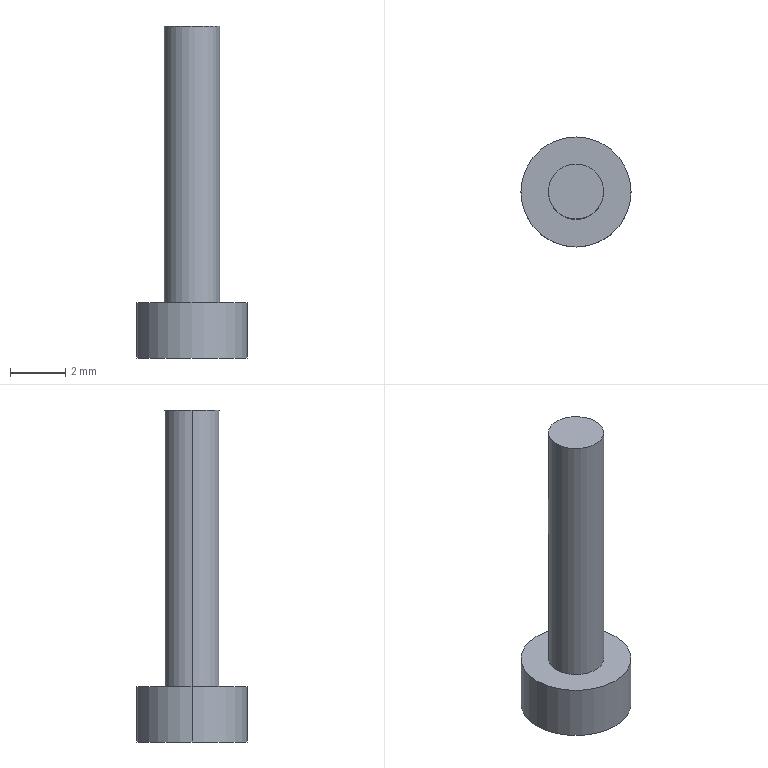Part | SolidWorks | features BaseBody 1 | 1 solid | 14 faces | box 3.98 x 3.98 x 12 mm | volume 54.19 mm3 | plane 10 | cylinder 4 | commonest cylinder face diameters 2 x2 3.98 x2
STEP:
#1=CARTESIAN_POINT('',(-1.,0.,12.));
#2=VERTEX_POINT('',#1);
#3=CARTESIAN_POINT('',(1.,0.,12.));
#4=VERTEX_POINT('',#3);
#5=CARTESIAN_POINT('',(0.,0.,12.));
#6=DIRECTION('',(0.,0.,-1.));
#7=DIRECTION('',(-1.,0.,0.));
#8=AXIS2_PLACEMENT_3D('',#5,#6,#7);
#9=CIRCLE('',#8,1.);
#10=EDGE_CURVE('',#2,#4,#9,.T.);
#11=ORIENTED_EDGE('',*,*,#10,.T.);
#12=CARTESIAN_POINT('',(1.,0.,2.));
#13=VERTEX_POINT('',#12);
#14=CARTESIAN_POINT('',(1.,0.,12.));
#15=DIRECTION('',(0.,0.,-1.));
#16=VECTOR('',#15,1000.);
#17=LINE('',#14,#16);
#18=EDGE_CURVE('',#4,#13,#17,.T.);
#19=ORIENTED_EDGE('',*,*,#18,.T.);
#20=CARTESIAN_POINT('',(-1.,0.,2.));
#21=VERTEX_POINT('',#20);
#22=CARTESIAN_POINT('',(0.,0.,2.));
#23=DIRECTION('',(0.,0.,1.));
#24=DIRECTION('',(-1.,0.,0.));
#25=AXIS2_PLACEMENT_3D('',#22,#23,#24);
#26=CIRCLE('',#25,1.);
#27=EDGE_CURVE('',#13,#21,#26,.T.);
#28=ORIENTED_EDGE('',*,*,#27,.T.);
#29=CARTESIAN_POINT('',(-1.,0.,12.));
#30=DIRECTION('',(0.,0.,-1.));
#31=VECTOR('',#30,1000.);
#32=LINE('',#29,#31);
#33=EDGE_CURVE('',#2,#21,#32,.T.);
#34=ORIENTED_EDGE('',*,*,#33,.F.);
#35=EDGE_LOOP('',(#11,#19,#28,#34));
#36=FACE_OUTER_BOUND('',#35,.T.);
#37=CARTESIAN_POINT('',(0.,0.,12.));
#38=DIRECTION('',(0.,0.,-1.));
#39=DIRECTION('',(-1.,0.,0.));
#40=AXIS2_PLACEMENT_3D('',#37,#38,#39);
#41=CYLINDRICAL_SURFACE('',#40,1.);
#42=ADVANCED_FACE('',(#36),#41,.T.);
#43=CARTESIAN_POINT('',(1.99,0.,2.));
#44=VERTEX_POINT('',#43);
#45=CARTESIAN_POINT('',(-1.99,0.,2.));
#46=VERTEX_POINT('',#45);
#47=CARTESIAN_POINT('',(0.,0.,2.));
#48=DIRECTION('',(0.,0.,1.));
#49=DIRECTION('',(-1.,0.,0.));
#50=AXIS2_PLACEMENT_3D('',#47,#48,#49);
#51=CIRCLE('',#50,1.99);
#52=EDGE_CURVE('',#44,#46,#51,.T.);
#53=ORIENTED_EDGE('',*,*,#52,.F.);
#54=CARTESIAN_POINT('',(1.99,0.,0.));
#55=VERTEX_POINT('',#54);
#56=CARTESIAN_POINT('',(1.99,0.,2.));
#57=DIRECTION('',(0.,0.,-1.));
#58=VECTOR('',#57,1000.);
#59=LINE('',#56,#58);
#60=EDGE_CURVE('',#44,#55,#59,.T.);
#61=ORIENTED_EDGE('',*,*,#60,.T.);
#62=CARTESIAN_POINT('',(-1.99,0.,0.));
#63=VERTEX_POINT('',#62);
#64=CARTESIAN_POINT('',(0.,0.,0.));
#65=DIRECTION('',(0.,0.,1.));
#66=DIRECTION('',(-1.,0.,0.));
#67=AXIS2_PLACEMENT_3D('',#64,#65,#66);
#68=CIRCLE('',#67,1.99);
#69=EDGE_CURVE('',#55,#63,#68,.T.);
#70=ORIENTED_EDGE('',*,*,#69,.T.);
#71=CARTESIAN_POINT('',(-1.99,0.,2.));
#72=DIRECTION('',(0.,0.,-1.));
#73=VECTOR('',#72,1000.);
#74=LINE('',#71,#73);
#75=EDGE_CURVE('',#46,#63,#74,.T.);
#76=ORIENTED_EDGE('',*,*,#75,.F.);
#77=EDGE_LOOP('',(#53,#61,#70,#76));
#78=FACE_OUTER_BOUND('',#77,.T.);
#79=CARTESIAN_POINT('',(0.,0.,2.));
#80=DIRECTION('',(0.,0.,-1.));
#81=DIRECTION('',(-1.,0.,0.));
#82=AXIS2_PLACEMENT_3D('',#79,#80,#81);
#83=CYLINDRICAL_SURFACE('',#82,1.99);
#84=ADVANCED_FACE('',(#78),#83,.T.);
#85=ORIENTED_EDGE('',*,*,#18,.F.);
#86=CARTESIAN_POINT('',(0.,0.,12.));
#87=DIRECTION('',(0.,0.,-1.));
#88=DIRECTION('',(-1.,0.,0.));
#89=AXIS2_PLACEMENT_3D('',#86,#87,#88);
#90=CIRCLE('',#89,1.);
#91=EDGE_CURVE('',#4,#2,#90,.T.);
#92=ORIENTED_EDGE('',*,*,#91,.T.);
#93=ORIENTED_EDGE('',*,*,#33,.T.);
#94=CARTESIAN_POINT('',(0.,0.,2.));
#95=DIRECTION('',(0.,0.,1.));
#96=DIRECTION('',(-1.,0.,0.));
#97=AXIS2_PLACEMENT_3D('',#94,#95,#96);
#98=CIRCLE('',#97,1.);
#99=EDGE_CURVE('',#21,#13,#98,.T.);
#100=ORIENTED_EDGE('',*,*,#99,.T.);
#101=EDGE_LOOP('',(#85,#92,#93,#100));
#102=FACE_OUTER_BOUND('',#101,.T.);
#103=CARTESIAN_POINT('',(0.,0.,12.));
#104=DIRECTION('',(0.,0.,-1.));
#105=DIRECTION('',(-1.,0.,0.));
#106=AXIS2_PLACEMENT_3D('',#103,#104,#105);
#107=CYLINDRICAL_SURFACE('',#106,1.);
#108=ADVANCED_FACE('',(#102),#107,.T.);
#109=CARTESIAN_POINT('',(0.,0.,2.));
#110=DIRECTION('',(0.,0.,1.));
#111=DIRECTION('',(-1.,0.,0.));
#112=AXIS2_PLACEMENT_3D('',#109,#110,#111);
#113=CIRCLE('',#112,1.99);
#114=EDGE_CURVE('',#46,#44,#113,.T.);
#115=ORIENTED_EDGE('',*,*,#114,.T.);
#116=ORIENTED_EDGE('',*,*,#52,.T.);
#117=EDGE_LOOP('',(#115,#116));
#118=FACE_OUTER_BOUND('',#117,.T.);
#119=ORIENTED_EDGE('',*,*,#99,.F.);
#120=ORIENTED_EDGE('',*,*,#27,.F.);
#121=EDGE_LOOP('',(#119,#120));
#122=FACE_BOUND('',#121,.T.);
#123=CARTESIAN_POINT('',(0.,0.,2.));
#124=DIRECTION('',(0.,0.,1.));
#125=DIRECTION('',(1.,0.,0.));
#126=AXIS2_PLACEMENT_3D('',#123,#124,#125);
#127=PLANE('',#126);
#128=ADVANCED_FACE('',(#118,#122),#127,.T.);
#129=ORIENTED_EDGE('',*,*,#10,.F.);
#130=ORIENTED_EDGE('',*,*,#91,.F.);
#131=EDGE_LOOP('',(#129,#130));
#132=FACE_OUTER_BOUND('',#131,.T.);
#133=CARTESIAN_POINT('',(0.,0.,12.));
#134=DIRECTION('',(0.,0.,1.));
#135=DIRECTION('',(1.,0.,0.));
#136=AXIS2_PLACEMENT_3D('',#133,#134,#135);
#137=PLANE('',#136);
#138=ADVANCED_FACE('',(#132),#137,.T.);
#139=ORIENTED_EDGE('',*,*,#60,.F.);
#140=ORIENTED_EDGE('',*,*,#114,.F.);
#141=ORIENTED_EDGE('',*,*,#75,.T.);
#142=CARTESIAN_POINT('',(0.,0.,0.));
#143=DIRECTION('',(0.,0.,1.));
#144=DIRECTION('',(-1.,0.,0.));
#145=AXIS2_PLACEMENT_3D('',#142,#143,#144);
#146=CIRCLE('',#145,1.99);
#147=EDGE_CURVE('',#63,#55,#146,.T.);
#148=ORIENTED_EDGE('',*,*,#147,.T.);
#149=EDGE_LOOP('',(#139,#140,#141,#148));
#150=FACE_OUTER_BOUND('',#149,.T.);
#151=CARTESIAN_POINT('',(0.,0.,2.));
#152=DIRECTION('',(0.,0.,-1.));
#153=DIRECTION('',(-1.,0.,0.));
#154=AXIS2_PLACEMENT_3D('',#151,#152,#153);
#155=CYLINDRICAL_SURFACE('',#154,1.99);
#156=ADVANCED_FACE('',(#150),#155,.T.);
#157=ORIENTED_EDGE('',*,*,#147,.F.);
#158=ORIENTED_EDGE('',*,*,#69,.F.);
#159=EDGE_LOOP('',(#157,#158));
#160=FACE_OUTER_BOUND('',#159,.T.);
#161=CARTESIAN_POINT('',(-0.78,0.4503,0.));
#162=VERTEX_POINT('',#161);
#163=CARTESIAN_POINT('',(0.,0.9007,0.));
#164=VERTEX_POINT('',#163);
#165=CARTESIAN_POINT('',(-0.78,0.4503,0.));
#166=DIRECTION('',(0.866,0.5,0.));
#167=VECTOR('',#166,1000.);
#168=LINE('',#165,#167);
#169=EDGE_CURVE('',#162,#164,#168,.T.);
#170=ORIENTED_EDGE('',*,*,#169,.F.);
#171=CARTESIAN_POINT('',(-0.78,-0.4503,0.));
#172=VERTEX_POINT('',#171);
#173=CARTESIAN_POINT('',(-0.78,0.,0.));
#174=DIRECTION('',(0.,1.,0.));
#175=VECTOR('',#174,1000.);
#176=LINE('',#173,#175);
#177=EDGE_CURVE('',#172,#162,#176,.T.);
#178=ORIENTED_EDGE('',*,*,#177,.F.);
#179=CARTESIAN_POINT('',(0.,-0.9007,0.));
#180=VERTEX_POINT('',#179);
#181=CARTESIAN_POINT('',(0.,-0.9007,0.));
#182=DIRECTION('',(-0.866,0.5,0.));
#183=VECTOR('',#182,1000.);
#184=LINE('',#181,#183);
#185=EDGE_CURVE('',#180,#172,#184,.T.);
#186=ORIENTED_EDGE('',*,*,#185,.F.);
#187=CARTESIAN_POINT('',(0.78,-0.4503,0.));
#188=VERTEX_POINT('',#187);
#189=CARTESIAN_POINT('',(0.78,-0.4503,0.));
#190=DIRECTION('',(-0.866,-0.5,0.));
#191=VECTOR('',#190,1000.);
#192=LINE('',#189,#191);
#193=EDGE_CURVE('',#188,#180,#192,.T.);
#194=ORIENTED_EDGE('',*,*,#193,.F.);
#195=CARTESIAN_POINT('',(0.78,0.4503,0.));
#196=VERTEX_POINT('',#195);
#197=CARTESIAN_POINT('',(0.78,0.,0.));
#198=DIRECTION('',(0.,-1.,0.));
#199=VECTOR('',#198,1000.);
#200=LINE('',#197,#199);
#201=EDGE_CURVE('',#196,#188,#200,.T.);
#202=ORIENTED_EDGE('',*,*,#201,.F.);
#203=CARTESIAN_POINT('',(0.,0.9007,0.));
#204=DIRECTION('',(0.866,-0.5,0.));
#205=VECTOR('',#204,1000.);
#206=LINE('',#203,#205);
#207=EDGE_CURVE('',#164,#196,#206,.T.);
#208=ORIENTED_EDGE('',*,*,#207,.F.);
#209=EDGE_LOOP('',(#170,#178,#186,#194,#202,#208));
#210=FACE_BOUND('',#209,.T.);
#211=CARTESIAN_POINT('',(0.,0.,0.));
#212=DIRECTION('',(0.,0.,1.));
#213=DIRECTION('',(1.,0.,0.));
#214=AXIS2_PLACEMENT_3D('',#211,#212,#213);
#215=PLANE('',#214);
#216=ADVANCED_FACE('',(#160,#210),#215,.F.);
#217=CARTESIAN_POINT('',(0.78,0.4503,1.));
#218=VERTEX_POINT('',#217);
#219=CARTESIAN_POINT('',(0.78,0.4503,1.));
#220=DIRECTION('',(0.,0.,-1.));
#221=VECTOR('',#220,1000.);
#222=LINE('',#219,#221);
#223=EDGE_CURVE('',#218,#196,#222,.T.);
#224=ORIENTED_EDGE('',*,*,#223,.F.);
#225=CARTESIAN_POINT('',(0.,0.9007,1.));
#226=VERTEX_POINT('',#225);
#227=CARTESIAN_POINT('',(0.,0.9007,1.));
#228=DIRECTION('',(0.866,-0.5,0.));
#229=VECTOR('',#228,1000.);
#230=LINE('',#227,#229);
#231=EDGE_CURVE('',#226,#218,#230,.T.);
#232=ORIENTED_EDGE('',*,*,#231,.F.);
#233=CARTESIAN_POINT('',(0.,0.9007,1.));
#234=DIRECTION('',(0.,0.,1.));
#235=VECTOR('',#234,1000.);
#236=LINE('',#233,#235);
#237=EDGE_CURVE('',#164,#226,#236,.T.);
#238=ORIENTED_EDGE('',*,*,#237,.F.);
#239=ORIENTED_EDGE('',*,*,#207,.T.);
#240=EDGE_LOOP('',(#224,#232,#238,#239));
#241=FACE_OUTER_BOUND('',#240,.T.);
#242=CARTESIAN_POINT('',(0.,0.9007,1.));
#243=DIRECTION('',(0.5,0.866,0.));
#244=DIRECTION('',(-0.866,0.5,0.));
#245=AXIS2_PLACEMENT_3D('',#242,#243,#244);
#246=PLANE('',#245);
#247=ADVANCED_FACE('',(#241),#246,.F.);
#248=ORIENTED_EDGE('',*,*,#237,.T.);
#249=CARTESIAN_POINT('',(-0.78,0.4503,1.));
#250=VERTEX_POINT('',#249);
#251=CARTESIAN_POINT('',(-0.78,0.4503,1.));
#252=DIRECTION('',(0.866,0.5,0.));
#253=VECTOR('',#252,1000.);
#254=LINE('',#251,#253);
#255=EDGE_CURVE('',#250,#226,#254,.T.);
#256=ORIENTED_EDGE('',*,*,#255,.F.);
#257=CARTESIAN_POINT('',(-0.78,0.4503,1.));
#258=DIRECTION('',(0.,0.,1.));
#259=VECTOR('',#258,1000.);
#260=LINE('',#257,#259);
#261=EDGE_CURVE('',#162,#250,#260,.T.);
#262=ORIENTED_EDGE('',*,*,#261,.F.);
#263=ORIENTED_EDGE('',*,*,#169,.T.);
#264=EDGE_LOOP('',(#248,#256,#262,#263));
#265=FACE_OUTER_BOUND('',#264,.T.);
#266=CARTESIAN_POINT('',(-0.78,0.4503,1.));
#267=DIRECTION('',(-0.5,0.866,0.));
#268=DIRECTION('',(-0.866,-0.5,0.));
#269=AXIS2_PLACEMENT_3D('',#266,#267,#268);
#270=PLANE('',#269);
#271=ADVANCED_FACE('',(#265),#270,.F.);
#272=ORIENTED_EDGE('',*,*,#261,.T.);
#273=CARTESIAN_POINT('',(-0.78,-0.4503,1.));
#274=VERTEX_POINT('',#273);
#275=CARTESIAN_POINT('',(-0.78,-0.4503,1.));
#276=DIRECTION('',(0.,1.,0.));
#277=VECTOR('',#276,1000.);
#278=LINE('',#275,#277);
#279=EDGE_CURVE('',#274,#250,#278,.T.);
#280=ORIENTED_EDGE('',*,*,#279,.F.);
#281=CARTESIAN_POINT('',(-0.78,-0.4503,1.));
#282=DIRECTION('',(0.,0.,1.));
#283=VECTOR('',#282,1000.);
#284=LINE('',#281,#283);
#285=EDGE_CURVE('',#172,#274,#284,.T.);
#286=ORIENTED_EDGE('',*,*,#285,.F.);
#287=ORIENTED_EDGE('',*,*,#177,.T.);
#288=EDGE_LOOP('',(#272,#280,#286,#287));
#289=FACE_OUTER_BOUND('',#288,.T.);
#290=CARTESIAN_POINT('',(-0.78,-0.4503,1.));
#291=DIRECTION('',(-1.,0.,0.));
#292=DIRECTION('',(0.,-1.,0.));
#293=AXIS2_PLACEMENT_3D('',#290,#291,#292);
#294=PLANE('',#293);
#295=ADVANCED_FACE('',(#289),#294,.F.);
#296=ORIENTED_EDGE('',*,*,#285,.T.);
#297=CARTESIAN_POINT('',(0.,-0.9007,1.));
#298=VERTEX_POINT('',#297);
#299=CARTESIAN_POINT('',(0.,-0.9007,1.));
#300=DIRECTION('',(-0.866,0.5,0.));
#301=VECTOR('',#300,1000.);
#302=LINE('',#299,#301);
#303=EDGE_CURVE('',#298,#274,#302,.T.);
#304=ORIENTED_EDGE('',*,*,#303,.F.);
#305=CARTESIAN_POINT('',(0.,-0.9007,1.));
#306=DIRECTION('',(0.,0.,1.));
#307=VECTOR('',#306,1000.);
#308=LINE('',#305,#307);
#309=EDGE_CURVE('',#180,#298,#308,.T.);
#310=ORIENTED_EDGE('',*,*,#309,.F.);
#311=ORIENTED_EDGE('',*,*,#185,.T.);
#312=EDGE_LOOP('',(#296,#304,#310,#311));
#313=FACE_OUTER_BOUND('',#312,.T.);
#314=CARTESIAN_POINT('',(0.,-0.9007,1.));
#315=DIRECTION('',(-0.5,-0.866,0.));
#316=DIRECTION('',(0.866,-0.5,0.));
#317=AXIS2_PLACEMENT_3D('',#314,#315,#316);
#318=PLANE('',#317);
#319=ADVANCED_FACE('',(#313),#318,.F.);
#320=ORIENTED_EDGE('',*,*,#309,.T.);
#321=CARTESIAN_POINT('',(0.78,-0.4503,1.));
#322=VERTEX_POINT('',#321);
#323=CARTESIAN_POINT('',(0.78,-0.4503,1.));
#324=DIRECTION('',(-0.866,-0.5,0.));
#325=VECTOR('',#324,1000.);
#326=LINE('',#323,#325);
#327=EDGE_CURVE('',#322,#298,#326,.T.);
#328=ORIENTED_EDGE('',*,*,#327,.F.);
#329=CARTESIAN_POINT('',(0.78,-0.4503,1.));
#330=DIRECTION('',(0.,0.,1.));
#331=VECTOR('',#330,1000.);
#332=LINE('',#329,#331);
#333=EDGE_CURVE('',#188,#322,#332,.T.);
#334=ORIENTED_EDGE('',*,*,#333,.F.);
#335=ORIENTED_EDGE('',*,*,#193,.T.);
#336=EDGE_LOOP('',(#320,#328,#334,#335));
#337=FACE_OUTER_BOUND('',#336,.T.);
#338=CARTESIAN_POINT('',(0.78,-0.4503,1.));
#339=DIRECTION('',(0.5,-0.866,0.));
#340=DIRECTION('',(0.866,0.5,0.));
#341=AXIS2_PLACEMENT_3D('',#338,#339,#340);
#342=PLANE('',#341);
#343=ADVANCED_FACE('',(#337),#342,.F.);
#344=ORIENTED_EDGE('',*,*,#333,.T.);
#345=CARTESIAN_POINT('',(0.78,0.4503,1.));
#346=DIRECTION('',(0.,-1.,0.));
#347=VECTOR('',#346,1000.);
#348=LINE('',#345,#347);
#349=EDGE_CURVE('',#218,#322,#348,.T.);
#350=ORIENTED_EDGE('',*,*,#349,.F.);
#351=ORIENTED_EDGE('',*,*,#223,.T.);
#352=ORIENTED_EDGE('',*,*,#201,.T.);
#353=EDGE_LOOP('',(#344,#350,#351,#352));
#354=FACE_OUTER_BOUND('',#353,.T.);
#355=CARTESIAN_POINT('',(0.78,0.4503,1.));
#356=DIRECTION('',(1.,0.,0.));
#357=DIRECTION('',(0.,1.,0.));
#358=AXIS2_PLACEMENT_3D('',#355,#356,#357);
#359=PLANE('',#358);
#360=ADVANCED_FACE('',(#354),#359,.F.);
#361=ORIENTED_EDGE('',*,*,#303,.T.);
#362=ORIENTED_EDGE('',*,*,#279,.T.);
#363=ORIENTED_EDGE('',*,*,#255,.T.);
#364=ORIENTED_EDGE('',*,*,#231,.T.);
#365=ORIENTED_EDGE('',*,*,#349,.T.);
#366=ORIENTED_EDGE('',*,*,#327,.T.);
#367=EDGE_LOOP('',(#361,#362,#363,#364,#365,#366));
#368=FACE_OUTER_BOUND('',#367,.T.);
#369=CARTESIAN_POINT('',(0.,0.,1.));
#370=DIRECTION('',(0.,0.,-1.));
#371=DIRECTION('',(-1.,0.,0.));
#372=AXIS2_PLACEMENT_3D('',#369,#370,#371);
#373=PLANE('',#372);
#374=ADVANCED_FACE('',(#368),#373,.T.);
#375=CLOSED_SHELL('',(#42,#84,#108,#128,#138,#156,#216,#247,#271,#295,#319,#343,#360,#374));
#376=MANIFOLD_SOLID_BREP('',#375);
#377=CARTESIAN_POINT('',(0.,0.,0.));
#378=DIRECTION('',(0.,0.,1.));
#379=DIRECTION('',(1.,0.,0.));
#380=AXIS2_PLACEMENT_3D('',#377,#378,#379);
#381=(LENGTH_UNIT()NAMED_UNIT(*)SI_UNIT(.MILLI.,.METRE.));
#382=UNCERTAINTY_MEASURE_WITH_UNIT(LENGTH_MEASURE(0.00001),#381,'','');
#383=(NAMED_UNIT(*)PLANE_ANGLE_UNIT()SI_UNIT($,.RADIAN.));
#384=(NAMED_UNIT(*)SI_UNIT($,.STERADIAN.)SOLID_ANGLE_UNIT());
#385=(GEOMETRIC_REPRESENTATION_CONTEXT(3)GLOBAL_UNCERTAINTY_ASSIGNED_CONTEXT((#382))GLOBAL_UNIT_ASSIGNED_CONTEXT((#381,#383,#384))REPRESENTATION_CONTEXT('',''));
#386=ADVANCED_BREP_SHAPE_REPRESENTATION('',(#376,#380),#385);